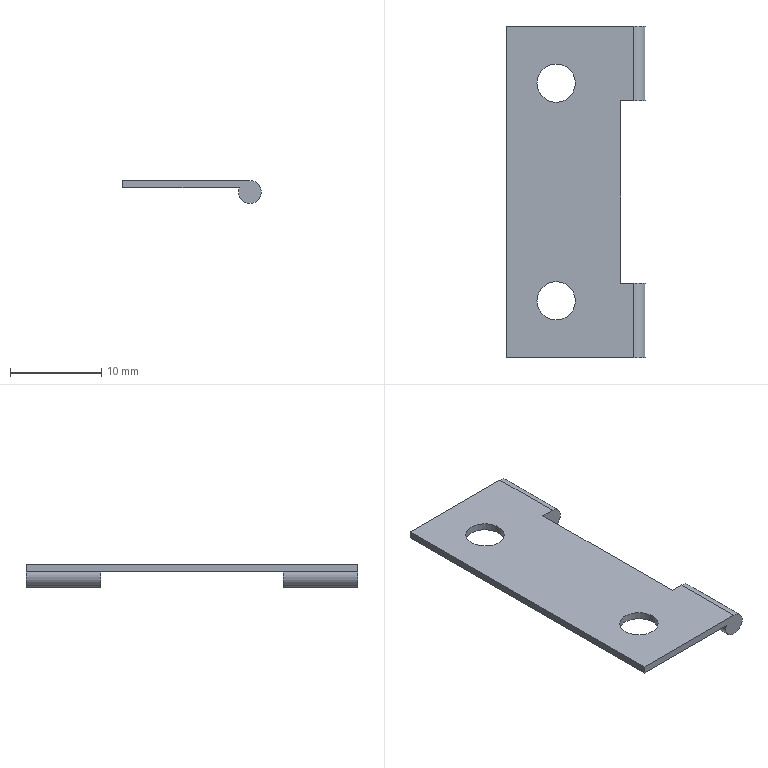Part | STEP file | 1.5 inch micro hinge plate-left | 1 solid | 16 faces | box 15.15 x 36.2 x 2.5 mm | volume 425.73 mm3 | cylinder 8 | plane 8 | commonest cylinder face diameters 2.5 x4 4.2 x4
STEP:
#1=CARTESIAN_POINT('',(0.,0.,0.));
#2=DIRECTION('',(0.,0.,1.));
#3=DIRECTION('',(1.,0.,0.));
#4=AXIS2_PLACEMENT_3D('',#1,#2,#3);
#5=CARTESIAN_POINT('',(-3.65,11.9,0.4));
#6=VERTEX_POINT('',#5);
#7=CARTESIAN_POINT('',(-3.65,11.9,-0.4));
#8=VERTEX_POINT('',#7);
#9=CARTESIAN_POINT('',(-3.65,11.9,-0.4));
#10=DIRECTION('',(0.,0.,-1.));
#11=VECTOR('',#10,1.);
#12=LINE('',#9,#11);
#13=CARTESIAN_POINT('',(-1.55,11.9,-0.4));
#14=DIRECTION('',(0.,0.,-1.));
#15=DIRECTION('',(-1.,0.,0.));
#16=AXIS2_PLACEMENT_3D('',#13,#14,#15);
#17=CYLINDRICAL_SURFACE('',#16,2.1);
#18=CARTESIAN_POINT('',(6.283,0.));
#19=DIRECTION('',(0.,1.));
#20=VECTOR('',#19,1.);
#21=LINE('',#18,#20);
#22=(GEOMETRIC_REPRESENTATION_CONTEXT(2)PARAMETRIC_REPRESENTATION_CONTEXT()REPRESENTATION_CONTEXT('',''));
#23=DEFINITIONAL_REPRESENTATION('',(#21),#22);
#24=PCURVE('',#17,#23);
#25=CARTESIAN_POINT('',(-1.55,11.9,-0.4));
#26=DIRECTION('',(0.,0.,-1.));
#27=DIRECTION('',(-1.,0.,0.));
#28=AXIS2_PLACEMENT_3D('',#25,#26,#27);
#29=CYLINDRICAL_SURFACE('',#28,2.1);
#30=CARTESIAN_POINT('',(0.,0.));
#31=DIRECTION('',(0.,1.));
#32=VECTOR('',#31,1.);
#33=LINE('',#30,#32);
#34=(GEOMETRIC_REPRESENTATION_CONTEXT(2)PARAMETRIC_REPRESENTATION_CONTEXT()REPRESENTATION_CONTEXT('',''));
#35=DEFINITIONAL_REPRESENTATION('',(#33),#34);
#36=PCURVE('',#29,#35);
#37=SURFACE_CURVE('',#12,(#24,#36),.PCURVE_S1.);
#38=EDGE_CURVE('',#6,#8,#37,.T.);
#39=ORIENTED_EDGE('',*,*,#38,.T.);
#40=CARTESIAN_POINT('',(0.55,11.9,-0.4));
#41=VERTEX_POINT('',#40);
#42=CARTESIAN_POINT('',(-1.55,11.9,-0.4));
#43=DIRECTION('',(0.,0.,-1.));
#44=DIRECTION('',(-1.,0.,0.));
#45=AXIS2_PLACEMENT_3D('',#42,#43,#44);
#46=CIRCLE('',#45,2.1);
#47=CARTESIAN_POINT('',(0.,0.));
#48=DIRECTION('',(1.,0.));
#49=VECTOR('',#48,1.);
#50=LINE('',#47,#49);
#51=(GEOMETRIC_REPRESENTATION_CONTEXT(2)PARAMETRIC_REPRESENTATION_CONTEXT()REPRESENTATION_CONTEXT('',''));
#52=DEFINITIONAL_REPRESENTATION('',(#50),#51);
#53=PCURVE('',#17,#52);
#54=CARTESIAN_POINT('',(0.,0.,-0.4));
#55=DIRECTION('',(0.,0.,-1.));
#56=DIRECTION('',(-1.,0.,0.));
#57=AXIS2_PLACEMENT_3D('',#54,#55,#56);
#58=PLANE('',#57);
#59=CARTESIAN_POINT('',(1.55,11.9));
#60=DIRECTION('',(1.,0.));
#61=AXIS2_PLACEMENT_2D('',#59,#60);
#62=CIRCLE('',#61,2.1);
#63=(GEOMETRIC_REPRESENTATION_CONTEXT(2)PARAMETRIC_REPRESENTATION_CONTEXT()REPRESENTATION_CONTEXT('',''));
#64=DEFINITIONAL_REPRESENTATION('',(#62),#63);
#65=PCURVE('',#58,#64);
#66=SURFACE_CURVE('',#46,(#53,#65),.PCURVE_S1.);
#67=EDGE_CURVE('',#41,#8,#66,.T.);
#68=ORIENTED_EDGE('',*,*,#67,.F.);
#69=CARTESIAN_POINT('',(0.55,11.9,0.4));
#70=VERTEX_POINT('',#69);
#71=CARTESIAN_POINT('',(0.55,11.9,-0.4));
#72=DIRECTION('',(0.,0.,-1.));
#73=VECTOR('',#72,1.);
#74=LINE('',#71,#73);
#75=CARTESIAN_POINT('',(3.142,0.));
#76=DIRECTION('',(0.,1.));
#77=VECTOR('',#76,1.);
#78=LINE('',#75,#77);
#79=(GEOMETRIC_REPRESENTATION_CONTEXT(2)PARAMETRIC_REPRESENTATION_CONTEXT()REPRESENTATION_CONTEXT('',''));
#80=DEFINITIONAL_REPRESENTATION('',(#78),#79);
#81=PCURVE('',#17,#80);
#82=CARTESIAN_POINT('',(3.142,0.));
#83=DIRECTION('',(0.,1.));
#84=VECTOR('',#83,1.);
#85=LINE('',#82,#84);
#86=(GEOMETRIC_REPRESENTATION_CONTEXT(2)PARAMETRIC_REPRESENTATION_CONTEXT()REPRESENTATION_CONTEXT('',''));
#87=DEFINITIONAL_REPRESENTATION('',(#85),#86);
#88=PCURVE('',#29,#87);
#89=SURFACE_CURVE('',#74,(#81,#88),.PCURVE_S1.);
#90=EDGE_CURVE('',#70,#41,#89,.T.);
#91=ORIENTED_EDGE('',*,*,#90,.F.);
#92=CARTESIAN_POINT('',(-1.55,11.9,0.4));
#93=DIRECTION('',(0.,0.,-1.));
#94=DIRECTION('',(-1.,0.,0.));
#95=AXIS2_PLACEMENT_3D('',#92,#93,#94);
#96=CIRCLE('',#95,2.1);
#97=CARTESIAN_POINT('',(0.,-0.8));
#98=DIRECTION('',(1.,0.));
#99=VECTOR('',#98,1.);
#100=LINE('',#97,#99);
#101=(GEOMETRIC_REPRESENTATION_CONTEXT(2)PARAMETRIC_REPRESENTATION_CONTEXT()REPRESENTATION_CONTEXT('',''));
#102=DEFINITIONAL_REPRESENTATION('',(#100),#101);
#103=PCURVE('',#17,#102);
#104=CARTESIAN_POINT('',(0.,0.,0.4));
#105=DIRECTION('',(0.,0.,-1.));
#106=DIRECTION('',(-1.,0.,0.));
#107=AXIS2_PLACEMENT_3D('',#104,#105,#106);
#108=PLANE('',#107);
#109=CARTESIAN_POINT('',(1.55,11.9));
#110=DIRECTION('',(1.,0.));
#111=AXIS2_PLACEMENT_2D('',#109,#110);
#112=CIRCLE('',#111,2.1);
#113=(GEOMETRIC_REPRESENTATION_CONTEXT(2)PARAMETRIC_REPRESENTATION_CONTEXT()REPRESENTATION_CONTEXT('',''));
#114=DEFINITIONAL_REPRESENTATION('',(#112),#113);
#115=PCURVE('',#108,#114);
#116=SURFACE_CURVE('',#96,(#103,#115),.PCURVE_S1.);
#117=EDGE_CURVE('',#70,#6,#116,.T.);
#118=ORIENTED_EDGE('',*,*,#117,.T.);
#119=EDGE_LOOP('',(#39,#68,#91,#118));
#120=FACE_BOUND('',#119,.F.);
#121=ADVANCED_FACE('',(#120),#17,.F.);
#122=CARTESIAN_POINT('',(-3.65,-11.9,0.4));
#123=VERTEX_POINT('',#122);
#124=CARTESIAN_POINT('',(-3.65,-11.9,-0.4));
#125=VERTEX_POINT('',#124);
#126=CARTESIAN_POINT('',(-3.65,-11.9,-0.4));
#127=DIRECTION('',(0.,0.,-1.));
#128=VECTOR('',#127,1.);
#129=LINE('',#126,#128);
#130=CARTESIAN_POINT('',(-1.55,-11.9,-0.4));
#131=DIRECTION('',(0.,0.,-1.));
#132=DIRECTION('',(-1.,0.,0.));
#133=AXIS2_PLACEMENT_3D('',#130,#131,#132);
#134=CYLINDRICAL_SURFACE('',#133,2.1);
#135=CARTESIAN_POINT('',(6.283,0.));
#136=DIRECTION('',(0.,1.));
#137=VECTOR('',#136,1.);
#138=LINE('',#135,#137);
#139=(GEOMETRIC_REPRESENTATION_CONTEXT(2)PARAMETRIC_REPRESENTATION_CONTEXT()REPRESENTATION_CONTEXT('',''));
#140=DEFINITIONAL_REPRESENTATION('',(#138),#139);
#141=PCURVE('',#134,#140);
#142=CARTESIAN_POINT('',(-1.55,-11.9,-0.4));
#143=DIRECTION('',(0.,0.,-1.));
#144=DIRECTION('',(-1.,0.,0.));
#145=AXIS2_PLACEMENT_3D('',#142,#143,#144);
#146=CYLINDRICAL_SURFACE('',#145,2.1);
#147=CARTESIAN_POINT('',(0.,0.));
#148=DIRECTION('',(0.,1.));
#149=VECTOR('',#148,1.);
#150=LINE('',#147,#149);
#151=(GEOMETRIC_REPRESENTATION_CONTEXT(2)PARAMETRIC_REPRESENTATION_CONTEXT()REPRESENTATION_CONTEXT('',''));
#152=DEFINITIONAL_REPRESENTATION('',(#150),#151);
#153=PCURVE('',#146,#152);
#154=SURFACE_CURVE('',#129,(#141,#153),.PCURVE_S1.);
#155=EDGE_CURVE('',#123,#125,#154,.T.);
#156=ORIENTED_EDGE('',*,*,#155,.T.);
#157=CARTESIAN_POINT('',(0.55,-11.9,-0.4));
#158=VERTEX_POINT('',#157);
#159=CARTESIAN_POINT('',(-1.55,-11.9,-0.4));
#160=DIRECTION('',(0.,0.,-1.));
#161=DIRECTION('',(-1.,0.,0.));
#162=AXIS2_PLACEMENT_3D('',#159,#160,#161);
#163=CIRCLE('',#162,2.1);
#164=CARTESIAN_POINT('',(0.,0.));
#165=DIRECTION('',(1.,0.));
#166=VECTOR('',#165,1.);
#167=LINE('',#164,#166);
#168=(GEOMETRIC_REPRESENTATION_CONTEXT(2)PARAMETRIC_REPRESENTATION_CONTEXT()REPRESENTATION_CONTEXT('',''));
#169=DEFINITIONAL_REPRESENTATION('',(#167),#168);
#170=PCURVE('',#134,#169);
#171=CARTESIAN_POINT('',(1.55,-11.9));
#172=DIRECTION('',(1.,0.));
#173=AXIS2_PLACEMENT_2D('',#171,#172);
#174=CIRCLE('',#173,2.1);
#175=(GEOMETRIC_REPRESENTATION_CONTEXT(2)PARAMETRIC_REPRESENTATION_CONTEXT()REPRESENTATION_CONTEXT('',''));
#176=DEFINITIONAL_REPRESENTATION('',(#174),#175);
#177=PCURVE('',#58,#176);
#178=SURFACE_CURVE('',#163,(#170,#177),.PCURVE_S1.);
#179=EDGE_CURVE('',#158,#125,#178,.T.);
#180=ORIENTED_EDGE('',*,*,#179,.F.);
#181=CARTESIAN_POINT('',(0.55,-11.9,0.4));
#182=VERTEX_POINT('',#181);
#183=CARTESIAN_POINT('',(0.55,-11.9,-0.4));
#184=DIRECTION('',(0.,0.,-1.));
#185=VECTOR('',#184,1.);
#186=LINE('',#183,#185);
#187=CARTESIAN_POINT('',(3.142,0.));
#188=DIRECTION('',(0.,1.));
#189=VECTOR('',#188,1.);
#190=LINE('',#187,#189);
#191=(GEOMETRIC_REPRESENTATION_CONTEXT(2)PARAMETRIC_REPRESENTATION_CONTEXT()REPRESENTATION_CONTEXT('',''));
#192=DEFINITIONAL_REPRESENTATION('',(#190),#191);
#193=PCURVE('',#134,#192);
#194=CARTESIAN_POINT('',(3.142,0.));
#195=DIRECTION('',(0.,1.));
#196=VECTOR('',#195,1.);
#197=LINE('',#194,#196);
#198=(GEOMETRIC_REPRESENTATION_CONTEXT(2)PARAMETRIC_REPRESENTATION_CONTEXT()REPRESENTATION_CONTEXT('',''));
#199=DEFINITIONAL_REPRESENTATION('',(#197),#198);
#200=PCURVE('',#146,#199);
#201=SURFACE_CURVE('',#186,(#193,#200),.PCURVE_S1.);
#202=EDGE_CURVE('',#182,#158,#201,.T.);
#203=ORIENTED_EDGE('',*,*,#202,.F.);
#204=CARTESIAN_POINT('',(-1.55,-11.9,0.4));
#205=DIRECTION('',(0.,0.,-1.));
#206=DIRECTION('',(-1.,0.,0.));
#207=AXIS2_PLACEMENT_3D('',#204,#205,#206);
#208=CIRCLE('',#207,2.1);
#209=CARTESIAN_POINT('',(0.,-0.8));
#210=DIRECTION('',(1.,0.));
#211=VECTOR('',#210,1.);
#212=LINE('',#209,#211);
#213=(GEOMETRIC_REPRESENTATION_CONTEXT(2)PARAMETRIC_REPRESENTATION_CONTEXT()REPRESENTATION_CONTEXT('',''));
#214=DEFINITIONAL_REPRESENTATION('',(#212),#213);
#215=PCURVE('',#134,#214);
#216=CARTESIAN_POINT('',(1.55,-11.9));
#217=DIRECTION('',(1.,0.));
#218=AXIS2_PLACEMENT_2D('',#216,#217);
#219=CIRCLE('',#218,2.1);
#220=(GEOMETRIC_REPRESENTATION_CONTEXT(2)PARAMETRIC_REPRESENTATION_CONTEXT()REPRESENTATION_CONTEXT('',''));
#221=DEFINITIONAL_REPRESENTATION('',(#219),#220);
#222=PCURVE('',#108,#221);
#223=SURFACE_CURVE('',#208,(#215,#222),.PCURVE_S1.);
#224=EDGE_CURVE('',#182,#123,#223,.T.);
#225=ORIENTED_EDGE('',*,*,#224,.T.);
#226=EDGE_LOOP('',(#156,#180,#203,#225));
#227=FACE_BOUND('',#226,.F.);
#228=ADVANCED_FACE('',(#227),#134,.F.);
#229=CARTESIAN_POINT('',(6.95,18.1,-2.1));
#230=VERTEX_POINT('',#229);
#231=CARTESIAN_POINT('',(5.784,18.1,-0.4));
#232=VERTEX_POINT('',#231);
#233=CARTESIAN_POINT('',(6.95,18.1,-0.85));
#234=DIRECTION('',(0.,1.,0.));
#235=DIRECTION('',(0.,0.,1.));
#236=AXIS2_PLACEMENT_3D('',#233,#234,#235);
#237=CIRCLE('',#236,1.25);
#238=CARTESIAN_POINT('',(6.95,18.1,-0.85));
#239=DIRECTION('',(0.,-1.,0.));
#240=DIRECTION('',(0.,0.,-1.));
#241=AXIS2_PLACEMENT_3D('',#238,#239,#240);
#242=CYLINDRICAL_SURFACE('',#241,1.25);
#243=CARTESIAN_POINT('',(9.425,0.));
#244=DIRECTION('',(-1.,0.));
#245=VECTOR('',#244,1.);
#246=LINE('',#243,#245);
#247=(GEOMETRIC_REPRESENTATION_CONTEXT(2)PARAMETRIC_REPRESENTATION_CONTEXT()REPRESENTATION_CONTEXT('',''));
#248=DEFINITIONAL_REPRESENTATION('',(#246),#247);
#249=PCURVE('',#242,#248);
#250=CARTESIAN_POINT('',(-6.95,18.1,0.4));
#251=DIRECTION('',(0.,-1.,0.));
#252=DIRECTION('',(0.,0.,-1.));
#253=AXIS2_PLACEMENT_3D('',#250,#251,#252);
#254=PLANE('',#253);
#255=CARTESIAN_POINT('',(0.,13.9));
#256=CARTESIAN_POINT('',(0.,16.065));
#257=CARTESIAN_POINT('',(1.875,14.983));
#258=CARTESIAN_POINT('',(3.75,13.9));
#259=CARTESIAN_POINT('',(1.875,12.817));
#260=CARTESIAN_POINT('',(0.,11.735));
#261=CARTESIAN_POINT('',(0.,13.9));
#262=(BOUNDED_CURVE()B_SPLINE_CURVE(2,(#255,#256,#257,#258,#259,#260,#261),.UNSPECIFIED.,.T.,.F.)B_SPLINE_CURVE_WITH_KNOTS((1,2,2,2,2,1),(-2.094,0.,2.094,4.189,6.283,8.378),.UNSPECIFIED.)CURVE()GEOMETRIC_REPRESENTATION_ITEM()RATIONAL_B_SPLINE_CURVE((1.,0.5,1.,0.5,1.,0.5,1.))REPRESENTATION_ITEM(''));
#263=(GEOMETRIC_REPRESENTATION_CONTEXT(2)PARAMETRIC_REPRESENTATION_CONTEXT()REPRESENTATION_CONTEXT('',''));
#264=DEFINITIONAL_REPRESENTATION('',(#262),#263);
#265=PCURVE('',#254,#264);
#266=SURFACE_CURVE('',#237,(#249,#265),.PCURVE_S1.);
#267=EDGE_CURVE('',#230,#232,#266,.T.);
#268=ORIENTED_EDGE('',*,*,#267,.F.);
#269=CARTESIAN_POINT('',(6.95,10.,-2.1));
#270=VERTEX_POINT('',#269);
#271=CARTESIAN_POINT('',(6.95,18.1,-2.1));
#272=DIRECTION('',(0.,-1.,0.));
#273=VECTOR('',#272,1.);
#274=LINE('',#271,#273);
#275=CARTESIAN_POINT('',(6.283,0.));
#276=DIRECTION('',(0.,1.));
#277=VECTOR('',#276,1.);
#278=LINE('',#275,#277);
#279=(GEOMETRIC_REPRESENTATION_CONTEXT(2)PARAMETRIC_REPRESENTATION_CONTEXT()REPRESENTATION_CONTEXT('',''));
#280=DEFINITIONAL_REPRESENTATION('',(#278),#279);
#281=PCURVE('',#242,#280);
#282=CARTESIAN_POINT('',(6.95,18.1,-0.85));
#283=DIRECTION('',(0.,-1.,0.));
#284=DIRECTION('',(0.,0.,-1.));
#285=AXIS2_PLACEMENT_3D('',#282,#283,#284);
#286=CYLINDRICAL_SURFACE('',#285,1.25);
#287=CARTESIAN_POINT('',(0.,0.));
#288=DIRECTION('',(0.,1.));
#289=VECTOR('',#288,1.);
#290=LINE('',#287,#289);
#291=(GEOMETRIC_REPRESENTATION_CONTEXT(2)PARAMETRIC_REPRESENTATION_CONTEXT()REPRESENTATION_CONTEXT('',''));
#292=DEFINITIONAL_REPRESENTATION('',(#290),#291);
#293=PCURVE('',#286,#292);
#294=SURFACE_CURVE('',#274,(#281,#293),.PCURVE_S1.);
#295=EDGE_CURVE('',#230,#270,#294,.T.);
#296=ORIENTED_EDGE('',*,*,#295,.T.);
#297=CARTESIAN_POINT('',(5.784,10.,-0.4));
#298=VERTEX_POINT('',#297);
#299=CARTESIAN_POINT('',(6.95,10.,-0.85));
#300=DIRECTION('',(0.,1.,0.));
#301=DIRECTION('',(0.,0.,1.));
#302=AXIS2_PLACEMENT_3D('',#299,#300,#301);
#303=CIRCLE('',#302,1.25);
#304=CARTESIAN_POINT('',(9.425,8.1));
#305=DIRECTION('',(-1.,0.));
#306=VECTOR('',#305,1.);
#307=LINE('',#304,#306);
#308=(GEOMETRIC_REPRESENTATION_CONTEXT(2)PARAMETRIC_REPRESENTATION_CONTEXT()REPRESENTATION_CONTEXT('',''));
#309=DEFINITIONAL_REPRESENTATION('',(#307),#308);
#310=PCURVE('',#242,#309);
#311=CARTESIAN_POINT('',(5.5,10.,0.4));
#312=DIRECTION('',(0.,1.,0.));
#313=DIRECTION('',(0.,0.,1.));
#314=AXIS2_PLACEMENT_3D('',#311,#312,#313);
#315=PLANE('',#314);
#316=CARTESIAN_POINT('',(-1.25,1.45));
#317=DIRECTION('',(1.,0.));
#318=AXIS2_PLACEMENT_2D('',#316,#317);
#319=CIRCLE('',#318,1.25);
#320=(GEOMETRIC_REPRESENTATION_CONTEXT(2)PARAMETRIC_REPRESENTATION_CONTEXT()REPRESENTATION_CONTEXT('',''));
#321=DEFINITIONAL_REPRESENTATION('',(#319),#320);
#322=PCURVE('',#315,#321);
#323=SURFACE_CURVE('',#303,(#310,#322),.PCURVE_S1.);
#324=EDGE_CURVE('',#270,#298,#323,.T.);
#325=ORIENTED_EDGE('',*,*,#324,.T.);
#326=CARTESIAN_POINT('',(5.784,18.1,-0.4));
#327=DIRECTION('',(0.,-1.,0.));
#328=VECTOR('',#327,1.);
#329=LINE('',#326,#328);
#330=CARTESIAN_POINT('',(4.344,0.));
#331=DIRECTION('',(0.,1.));
#332=VECTOR('',#331,1.);
#333=LINE('',#330,#332);
#334=(GEOMETRIC_REPRESENTATION_CONTEXT(2)PARAMETRIC_REPRESENTATION_CONTEXT()REPRESENTATION_CONTEXT('',''));
#335=DEFINITIONAL_REPRESENTATION('',(#333),#334);
#336=PCURVE('',#242,#335);
#337=CARTESIAN_POINT('',(-5.784,18.1));
#338=DIRECTION('',(0.,-1.));
#339=VECTOR('',#338,1.);
#340=LINE('',#337,#339);
#341=(GEOMETRIC_REPRESENTATION_CONTEXT(2)PARAMETRIC_REPRESENTATION_CONTEXT()REPRESENTATION_CONTEXT('',''));
#342=DEFINITIONAL_REPRESENTATION('',(#340),#341);
#343=PCURVE('',#58,#342);
#344=SURFACE_CURVE('',#329,(#336,#343),.PCURVE_S1.);
#345=EDGE_CURVE('',#232,#298,#344,.T.);
#346=ORIENTED_EDGE('',*,*,#345,.F.);
#347=EDGE_LOOP('',(#268,#296,#325,#346));
#348=FACE_BOUND('',#347,.T.);
#349=ADVANCED_FACE('',(#348),#242,.T.);
#350=CARTESIAN_POINT('',(5.784,-10.,-0.4));
#351=VERTEX_POINT('',#350);
#352=CARTESIAN_POINT('',(6.95,-10.,-2.1));
#353=VERTEX_POINT('',#352);
#354=CARTESIAN_POINT('',(6.95,-10.,-0.85));
#355=DIRECTION('',(0.,-1.,0.));
#356=DIRECTION('',(0.,0.,-1.));
#357=AXIS2_PLACEMENT_3D('',#354,#355,#356);
#358=CIRCLE('',#357,1.25);
#359=CARTESIAN_POINT('',(6.95,18.1,-0.85));
#360=DIRECTION('',(0.,-1.,0.));
#361=DIRECTION('',(0.,0.,-1.));
#362=AXIS2_PLACEMENT_3D('',#359,#360,#361);
#363=CYLINDRICAL_SURFACE('',#362,1.25);
#364=CARTESIAN_POINT('',(0.,28.1));
#365=DIRECTION('',(1.,0.));
#366=VECTOR('',#365,1.);
#367=LINE('',#364,#366);
#368=(GEOMETRIC_REPRESENTATION_CONTEXT(2)PARAMETRIC_REPRESENTATION_CONTEXT()REPRESENTATION_CONTEXT('',''));
#369=DEFINITIONAL_REPRESENTATION('',(#367),#368);
#370=PCURVE('',#363,#369);
#371=CARTESIAN_POINT('',(5.5,-10.,0.4));
#372=DIRECTION('',(0.,-1.,0.));
#373=DIRECTION('',(0.,0.,-1.));
#374=AXIS2_PLACEMENT_3D('',#371,#372,#373);
#375=PLANE('',#374);
#376=CARTESIAN_POINT('',(1.25,1.45));
#377=DIRECTION('',(1.,0.));
#378=AXIS2_PLACEMENT_2D('',#376,#377);
#379=CIRCLE('',#378,1.25);
#380=(GEOMETRIC_REPRESENTATION_CONTEXT(2)PARAMETRIC_REPRESENTATION_CONTEXT()REPRESENTATION_CONTEXT('',''));
#381=DEFINITIONAL_REPRESENTATION('',(#379),#380);
#382=PCURVE('',#375,#381);
#383=SURFACE_CURVE('',#358,(#370,#382),.PCURVE_S1.);
#384=EDGE_CURVE('',#351,#353,#383,.T.);
#385=ORIENTED_EDGE('',*,*,#384,.T.);
#386=CARTESIAN_POINT('',(6.95,-18.1,-2.1));
#387=VERTEX_POINT('',#386);
#388=CARTESIAN_POINT('',(6.95,18.1,-2.1));
#389=DIRECTION('',(0.,-1.,0.));
#390=VECTOR('',#389,1.);
#391=LINE('',#388,#390);
#392=CARTESIAN_POINT('',(6.283,0.));
#393=DIRECTION('',(0.,1.));
#394=VECTOR('',#393,1.);
#395=LINE('',#392,#394);
#396=(GEOMETRIC_REPRESENTATION_CONTEXT(2)PARAMETRIC_REPRESENTATION_CONTEXT()REPRESENTATION_CONTEXT('',''));
#397=DEFINITIONAL_REPRESENTATION('',(#395),#396);
#398=PCURVE('',#363,#397);
#399=CARTESIAN_POINT('',(6.95,18.1,-0.85));
#400=DIRECTION('',(0.,-1.,0.));
#401=DIRECTION('',(0.,0.,-1.));
#402=AXIS2_PLACEMENT_3D('',#399,#400,#401);
#403=CYLINDRICAL_SURFACE('',#402,1.25);
#404=CARTESIAN_POINT('',(0.,0.));
#405=DIRECTION('',(0.,1.));
#406=VECTOR('',#405,1.);
#407=LINE('',#404,#406);
#408=(GEOMETRIC_REPRESENTATION_CONTEXT(2)PARAMETRIC_REPRESENTATION_CONTEXT()REPRESENTATION_CONTEXT('',''));
#409=DEFINITIONAL_REPRESENTATION('',(#407),#408);
#410=PCURVE('',#403,#409);
#411=SURFACE_CURVE('',#391,(#398,#410),.PCURVE_S1.);
#412=EDGE_CURVE('',#353,#387,#411,.T.);
#413=ORIENTED_EDGE('',*,*,#412,.T.);
#414=CARTESIAN_POINT('',(5.784,-18.1,-0.4));
#415=VERTEX_POINT('',#414);
#416=CARTESIAN_POINT('',(6.95,-18.1,-0.85));
#417=DIRECTION('',(0.,1.,0.));
#418=DIRECTION('',(0.,0.,1.));
#419=AXIS2_PLACEMENT_3D('',#416,#417,#418);
#420=CIRCLE('',#419,1.25);
#421=CARTESIAN_POINT('',(9.425,36.2));
#422=DIRECTION('',(-1.,0.));
#423=VECTOR('',#422,1.);
#424=LINE('',#421,#423);
#425=(GEOMETRIC_REPRESENTATION_CONTEXT(2)PARAMETRIC_REPRESENTATION_CONTEXT()REPRESENTATION_CONTEXT('',''));
#426=DEFINITIONAL_REPRESENTATION('',(#424),#425);
#427=PCURVE('',#363,#426);
#428=CARTESIAN_POINT('',(-6.95,-18.1,0.4));
#429=DIRECTION('',(0.,1.,0.));
#430=DIRECTION('',(0.,0.,1.));
#431=AXIS2_PLACEMENT_3D('',#428,#429,#430);
#432=PLANE('',#431);
#433=CARTESIAN_POINT('',(-1.25,13.9));
#434=DIRECTION('',(1.,0.));
#435=AXIS2_PLACEMENT_2D('',#433,#434);
#436=CIRCLE('',#435,1.25);
#437=(GEOMETRIC_REPRESENTATION_CONTEXT(2)PARAMETRIC_REPRESENTATION_CONTEXT()REPRESENTATION_CONTEXT('',''));
#438=DEFINITIONAL_REPRESENTATION('',(#436),#437);
#439=PCURVE('',#432,#438);
#440=SURFACE_CURVE('',#420,(#427,#439),.PCURVE_S1.);
#441=EDGE_CURVE('',#387,#415,#440,.T.);
#442=ORIENTED_EDGE('',*,*,#441,.T.);
#443=CARTESIAN_POINT('',(5.784,18.1,-0.4));
#444=DIRECTION('',(0.,-1.,0.));
#445=VECTOR('',#444,1.);
#446=LINE('',#443,#445);
#447=CARTESIAN_POINT('',(4.344,0.));
#448=DIRECTION('',(0.,1.));
#449=VECTOR('',#448,1.);
#450=LINE('',#447,#449);
#451=(GEOMETRIC_REPRESENTATION_CONTEXT(2)PARAMETRIC_REPRESENTATION_CONTEXT()REPRESENTATION_CONTEXT('',''));
#452=DEFINITIONAL_REPRESENTATION('',(#450),#451);
#453=PCURVE('',#363,#452);
#454=CARTESIAN_POINT('',(-5.784,18.1));
#455=DIRECTION('',(0.,-1.));
#456=VECTOR('',#455,1.);
#457=LINE('',#454,#456);
#458=(GEOMETRIC_REPRESENTATION_CONTEXT(2)PARAMETRIC_REPRESENTATION_CONTEXT()REPRESENTATION_CONTEXT('',''));
#459=DEFINITIONAL_REPRESENTATION('',(#457),#458);
#460=PCURVE('',#58,#459);
#461=SURFACE_CURVE('',#446,(#453,#460),.PCURVE_S1.);
#462=EDGE_CURVE('',#351,#415,#461,.T.);
#463=ORIENTED_EDGE('',*,*,#462,.F.);
#464=EDGE_LOOP('',(#385,#413,#442,#463));
#465=FACE_BOUND('',#464,.T.);
#466=ADVANCED_FACE('',(#465),#363,.T.);
#467=ORIENTED_EDGE('',*,*,#412,.F.);
#468=CARTESIAN_POINT('',(6.95,-10.,0.4));
#469=VERTEX_POINT('',#468);
#470=CARTESIAN_POINT('',(6.95,-10.,-0.85));
#471=DIRECTION('',(0.,-1.,0.));
#472=DIRECTION('',(0.,0.,-1.));
#473=AXIS2_PLACEMENT_3D('',#470,#471,#472);
#474=CIRCLE('',#473,1.25);
#475=CARTESIAN_POINT('',(0.,28.1));
#476=DIRECTION('',(1.,0.));
#477=VECTOR('',#476,1.);
#478=LINE('',#475,#477);
#479=(GEOMETRIC_REPRESENTATION_CONTEXT(2)PARAMETRIC_REPRESENTATION_CONTEXT()REPRESENTATION_CONTEXT('',''));
#480=DEFINITIONAL_REPRESENTATION('',(#478),#479);
#481=PCURVE('',#403,#480);
#482=CARTESIAN_POINT('',(1.25,1.45));
#483=DIRECTION('',(1.,0.));
#484=AXIS2_PLACEMENT_2D('',#482,#483);
#485=CIRCLE('',#484,1.25);
#486=(GEOMETRIC_REPRESENTATION_CONTEXT(2)PARAMETRIC_REPRESENTATION_CONTEXT()REPRESENTATION_CONTEXT('',''));
#487=DEFINITIONAL_REPRESENTATION('',(#485),#486);
#488=PCURVE('',#375,#487);
#489=SURFACE_CURVE('',#474,(#481,#488),.PCURVE_S1.);
#490=EDGE_CURVE('',#353,#469,#489,.T.);
#491=ORIENTED_EDGE('',*,*,#490,.T.);
#492=CARTESIAN_POINT('',(6.95,-18.1,0.4));
#493=VERTEX_POINT('',#492);
#494=CARTESIAN_POINT('',(6.95,-18.1,0.4));
#495=DIRECTION('',(0.,1.,0.));
#496=VECTOR('',#495,1.);
#497=LINE('',#494,#496);
#498=CARTESIAN_POINT('',(3.142,36.2));
#499=DIRECTION('',(0.,-1.));
#500=VECTOR('',#499,1.);
#501=LINE('',#498,#500);
#502=(GEOMETRIC_REPRESENTATION_CONTEXT(2)PARAMETRIC_REPRESENTATION_CONTEXT()REPRESENTATION_CONTEXT('',''));
#503=DEFINITIONAL_REPRESENTATION('',(#501),#502);
#504=PCURVE('',#403,#503);
#505=CARTESIAN_POINT('',(-6.95,-18.1));
#506=DIRECTION('',(0.,1.));
#507=VECTOR('',#506,1.);
#508=LINE('',#505,#507);
#509=(GEOMETRIC_REPRESENTATION_CONTEXT(2)PARAMETRIC_REPRESENTATION_CONTEXT()REPRESENTATION_CONTEXT('',''));
#510=DEFINITIONAL_REPRESENTATION('',(#508),#509);
#511=PCURVE('',#108,#510);
#512=SURFACE_CURVE('',#497,(#504,#511),.PCURVE_S1.);
#513=EDGE_CURVE('',#493,#469,#512,.T.);
#514=ORIENTED_EDGE('',*,*,#513,.F.);
#515=CARTESIAN_POINT('',(6.95,-18.1,-0.85));
#516=DIRECTION('',(0.,1.,0.));
#517=DIRECTION('',(0.,0.,1.));
#518=AXIS2_PLACEMENT_3D('',#515,#516,#517);
#519=CIRCLE('',#518,1.25);
#520=CARTESIAN_POINT('',(3.142,36.2));
#521=DIRECTION('',(-1.,0.));
#522=VECTOR('',#521,1.);
#523=LINE('',#520,#522);
#524=(GEOMETRIC_REPRESENTATION_CONTEXT(2)PARAMETRIC_REPRESENTATION_CONTEXT()REPRESENTATION_CONTEXT('',''));
#525=DEFINITIONAL_REPRESENTATION('',(#523),#524);
#526=PCURVE('',#403,#525);
#527=CARTESIAN_POINT('',(-1.25,13.9));
#528=DIRECTION('',(1.,0.));
#529=AXIS2_PLACEMENT_2D('',#527,#528);
#530=CIRCLE('',#529,1.25);
#531=(GEOMETRIC_REPRESENTATION_CONTEXT(2)PARAMETRIC_REPRESENTATION_CONTEXT()REPRESENTATION_CONTEXT('',''));
#532=DEFINITIONAL_REPRESENTATION('',(#530),#531);
#533=PCURVE('',#432,#532);
#534=SURFACE_CURVE('',#519,(#526,#533),.PCURVE_S1.);
#535=EDGE_CURVE('',#493,#387,#534,.T.);
#536=ORIENTED_EDGE('',*,*,#535,.T.);
#537=EDGE_LOOP('',(#467,#491,#514,#536));
#538=FACE_BOUND('',#537,.T.);
#539=ADVANCED_FACE('',(#538),#403,.T.);
#540=CARTESIAN_POINT('',(5.5,-10.,-0.4));
#541=VERTEX_POINT('',#540);
#542=CARTESIAN_POINT('',(0.,-10.,-0.4));
#543=DIRECTION('',(-1.,0.,0.));
#544=VECTOR('',#543,1.);
#545=LINE('',#542,#544);
#546=CARTESIAN_POINT('',(0.,-10.));
#547=DIRECTION('',(1.,0.));
#548=VECTOR('',#547,1.);
#549=LINE('',#546,#548);
#550=(GEOMETRIC_REPRESENTATION_CONTEXT(2)PARAMETRIC_REPRESENTATION_CONTEXT()REPRESENTATION_CONTEXT('',''));
#551=DEFINITIONAL_REPRESENTATION('',(#549),#550);
#552=PCURVE('',#58,#551);
#553=CARTESIAN_POINT('',(0.8,-5.5));
#554=DIRECTION('',(0.,-1.));
#555=VECTOR('',#554,1.);
#556=LINE('',#553,#555);
#557=(GEOMETRIC_REPRESENTATION_CONTEXT(2)PARAMETRIC_REPRESENTATION_CONTEXT()REPRESENTATION_CONTEXT('',''));
#558=DEFINITIONAL_REPRESENTATION('',(#556),#557);
#559=PCURVE('',#375,#558);
#560=SURFACE_CURVE('',#545,(#552,#559),.PCURVE_S1.);
#561=EDGE_CURVE('',#351,#541,#560,.T.);
#562=ORIENTED_EDGE('',*,*,#561,.F.);
#563=ORIENTED_EDGE('',*,*,#462,.T.);
#564=CARTESIAN_POINT('',(-6.95,-18.1,-0.4));
#565=VERTEX_POINT('',#564);
#566=CARTESIAN_POINT('',(-6.95,-18.1,-0.4));
#567=DIRECTION('',(1.,0.,0.));
#568=VECTOR('',#567,1.);
#569=LINE('',#566,#568);
#570=CARTESIAN_POINT('',(6.95,-18.1));
#571=DIRECTION('',(-1.,0.));
#572=VECTOR('',#571,1.);
#573=LINE('',#570,#572);
#574=(GEOMETRIC_REPRESENTATION_CONTEXT(2)PARAMETRIC_REPRESENTATION_CONTEXT()REPRESENTATION_CONTEXT('',''));
#575=DEFINITIONAL_REPRESENTATION('',(#573),#574);
#576=PCURVE('',#58,#575);
#577=CARTESIAN_POINT('',(-0.8,0.));
#578=DIRECTION('',(0.,1.));
#579=VECTOR('',#578,1.);
#580=LINE('',#577,#579);
#581=(GEOMETRIC_REPRESENTATION_CONTEXT(2)PARAMETRIC_REPRESENTATION_CONTEXT()REPRESENTATION_CONTEXT('',''));
#582=DEFINITIONAL_REPRESENTATION('',(#580),#581);
#583=PCURVE('',#432,#582);
#584=SURFACE_CURVE('',#569,(#576,#583),.PCURVE_S1.);
#585=EDGE_CURVE('',#565,#415,#584,.T.);
#586=ORIENTED_EDGE('',*,*,#585,.F.);
#587=CARTESIAN_POINT('',(-6.95,18.1,-0.4));
#588=VERTEX_POINT('',#587);
#589=CARTESIAN_POINT('',(-6.95,-18.1,-0.4));
#590=DIRECTION('',(0.,-1.,0.));
#591=VECTOR('',#590,1.);
#592=LINE('',#589,#591);
#593=CARTESIAN_POINT('',(6.95,-18.1));
#594=DIRECTION('',(0.,-1.));
#595=VECTOR('',#594,1.);
#596=LINE('',#593,#595);
#597=(GEOMETRIC_REPRESENTATION_CONTEXT(2)PARAMETRIC_REPRESENTATION_CONTEXT()REPRESENTATION_CONTEXT('',''));
#598=DEFINITIONAL_REPRESENTATION('',(#596),#597);
#599=PCURVE('',#58,#598);
#600=CARTESIAN_POINT('',(-6.95,-18.1,0.4));
#601=DIRECTION('',(1.,0.,0.));
#602=DIRECTION('',(0.,0.,-1.));
#603=AXIS2_PLACEMENT_3D('',#600,#601,#602);
#604=PLANE('',#603);
#605=CARTESIAN_POINT('',(0.8,0.));
#606=DIRECTION('',(0.,-1.));
#607=VECTOR('',#606,1.);
#608=LINE('',#605,#607);
#609=(GEOMETRIC_REPRESENTATION_CONTEXT(2)PARAMETRIC_REPRESENTATION_CONTEXT()REPRESENTATION_CONTEXT('',''));
#610=DEFINITIONAL_REPRESENTATION('',(#608),#609);
#611=PCURVE('',#604,#610);
#612=SURFACE_CURVE('',#592,(#599,#611),.PCURVE_S1.);
#613=EDGE_CURVE('',#588,#565,#612,.T.);
#614=ORIENTED_EDGE('',*,*,#613,.F.);
#615=CARTESIAN_POINT('',(-6.95,18.1,-0.4));
#616=DIRECTION('',(-1.,0.,0.));
#617=VECTOR('',#616,1.);
#618=LINE('',#615,#617);
#619=CARTESIAN_POINT('',(6.95,18.1));
#620=DIRECTION('',(1.,0.));
#621=VECTOR('',#620,1.);
#622=LINE('',#619,#621);
#623=(GEOMETRIC_REPRESENTATION_CONTEXT(2)PARAMETRIC_REPRESENTATION_CONTEXT()REPRESENTATION_CONTEXT('',''));
#624=DEFINITIONAL_REPRESENTATION('',(#622),#623);
#625=PCURVE('',#58,#624);
#626=CARTESIAN_POINT('',(0.8,0.));
#627=DIRECTION('',(0.,-1.));
#628=VECTOR('',#627,1.);
#629=LINE('',#626,#628);
#630=(GEOMETRIC_REPRESENTATION_CONTEXT(2)PARAMETRIC_REPRESENTATION_CONTEXT()REPRESENTATION_CONTEXT('',''));
#631=DEFINITIONAL_REPRESENTATION('',(#629),#630);
#632=PCURVE('',#254,#631);
#633=SURFACE_CURVE('',#618,(#625,#632),.PCURVE_S1.);
#634=EDGE_CURVE('',#232,#588,#633,.T.);
#635=ORIENTED_EDGE('',*,*,#634,.F.);
#636=ORIENTED_EDGE('',*,*,#345,.T.);
#637=CARTESIAN_POINT('',(5.5,10.,-0.4));
#638=VERTEX_POINT('',#637);
#639=CARTESIAN_POINT('',(0.,10.,-0.4));
#640=DIRECTION('',(1.,0.,0.));
#641=VECTOR('',#640,1.);
#642=LINE('',#639,#641);
#643=CARTESIAN_POINT('',(0.,10.));
#644=DIRECTION('',(-1.,0.));
#645=VECTOR('',#644,1.);
#646=LINE('',#643,#645);
#647=(GEOMETRIC_REPRESENTATION_CONTEXT(2)PARAMETRIC_REPRESENTATION_CONTEXT()REPRESENTATION_CONTEXT('',''));
#648=DEFINITIONAL_REPRESENTATION('',(#646),#647);
#649=PCURVE('',#58,#648);
#650=CARTESIAN_POINT('',(-0.8,-5.5));
#651=DIRECTION('',(0.,1.));
#652=VECTOR('',#651,1.);
#653=LINE('',#650,#652);
#654=(GEOMETRIC_REPRESENTATION_CONTEXT(2)PARAMETRIC_REPRESENTATION_CONTEXT()REPRESENTATION_CONTEXT('',''));
#655=DEFINITIONAL_REPRESENTATION('',(#653),#654);
#656=PCURVE('',#315,#655);
#657=SURFACE_CURVE('',#642,(#649,#656),.PCURVE_S1.);
#658=EDGE_CURVE('',#638,#298,#657,.T.);
#659=ORIENTED_EDGE('',*,*,#658,.F.);
#660=CARTESIAN_POINT('',(5.5,0.,-0.4));
#661=DIRECTION('',(0.,1.,0.));
#662=VECTOR('',#661,1.);
#663=LINE('',#660,#662);
#664=CARTESIAN_POINT('',(-5.5,0.));
#665=DIRECTION('',(0.,1.));
#666=VECTOR('',#665,1.);
#667=LINE('',#664,#666);
#668=(GEOMETRIC_REPRESENTATION_CONTEXT(2)PARAMETRIC_REPRESENTATION_CONTEXT()REPRESENTATION_CONTEXT('',''));
#669=DEFINITIONAL_REPRESENTATION('',(#667),#668);
#670=PCURVE('',#58,#669);
#671=CARTESIAN_POINT('',(5.5,0.,0.));
#672=DIRECTION('',(-1.,0.,0.));
#673=DIRECTION('',(0.,0.,1.));
#674=AXIS2_PLACEMENT_3D('',#671,#672,#673);
#675=PLANE('',#674);
#676=CARTESIAN_POINT('',(-0.4,0.));
#677=DIRECTION('',(0.,1.));
#678=VECTOR('',#677,1.);
#679=LINE('',#676,#678);
#680=(GEOMETRIC_REPRESENTATION_CONTEXT(2)PARAMETRIC_REPRESENTATION_CONTEXT()REPRESENTATION_CONTEXT('',''));
#681=DEFINITIONAL_REPRESENTATION('',(#679),#680);
#682=PCURVE('',#675,#681);
#683=SURFACE_CURVE('',#663,(#670,#682),.PCURVE_S1.);
#684=EDGE_CURVE('',#541,#638,#683,.T.);
#685=ORIENTED_EDGE('',*,*,#684,.F.);
#686=EDGE_LOOP('',(#562,#563,#586,#614,#635,#636,#659,#685));
#687=FACE_BOUND('',#686,.T.);
#688=CARTESIAN_POINT('',(-1.55,11.9,-0.4));
#689=DIRECTION('',(0.,0.,-1.));
#690=DIRECTION('',(-1.,0.,0.));
#691=AXIS2_PLACEMENT_3D('',#688,#689,#690);
#692=CIRCLE('',#691,2.1);
#693=CARTESIAN_POINT('',(1.55,11.9));
#694=DIRECTION('',(1.,0.));
#695=AXIS2_PLACEMENT_2D('',#693,#694);
#696=CIRCLE('',#695,2.1);
#697=(GEOMETRIC_REPRESENTATION_CONTEXT(2)PARAMETRIC_REPRESENTATION_CONTEXT()REPRESENTATION_CONTEXT('',''));
#698=DEFINITIONAL_REPRESENTATION('',(#696),#697);
#699=PCURVE('',#58,#698);
#700=CARTESIAN_POINT('',(0.,0.));
#701=DIRECTION('',(1.,0.));
#702=VECTOR('',#701,1.);
#703=LINE('',#700,#702);
#704=(GEOMETRIC_REPRESENTATION_CONTEXT(2)PARAMETRIC_REPRESENTATION_CONTEXT()REPRESENTATION_CONTEXT('',''));
#705=DEFINITIONAL_REPRESENTATION('',(#703),#704);
#706=PCURVE('',#29,#705);
#707=SURFACE_CURVE('',#692,(#699,#706),.PCURVE_S1.);
#708=EDGE_CURVE('',#8,#41,#707,.T.);
#709=ORIENTED_EDGE('',*,*,#708,.F.);
#710=ORIENTED_EDGE('',*,*,#67,.F.);
#711=EDGE_LOOP('',(#709,#710));
#712=FACE_BOUND('',#711,.T.);
#713=CARTESIAN_POINT('',(-1.55,-11.9,-0.4));
#714=DIRECTION('',(0.,0.,-1.));
#715=DIRECTION('',(-1.,0.,0.));
#716=AXIS2_PLACEMENT_3D('',#713,#714,#715);
#717=CIRCLE('',#716,2.1);
#718=CARTESIAN_POINT('',(1.55,-11.9));
#719=DIRECTION('',(1.,0.));
#720=AXIS2_PLACEMENT_2D('',#718,#719);
#721=CIRCLE('',#720,2.1);
#722=(GEOMETRIC_REPRESENTATION_CONTEXT(2)PARAMETRIC_REPRESENTATION_CONTEXT()REPRESENTATION_CONTEXT('',''));
#723=DEFINITIONAL_REPRESENTATION('',(#721),#722);
#724=PCURVE('',#58,#723);
#725=CARTESIAN_POINT('',(0.,0.));
#726=DIRECTION('',(1.,0.));
#727=VECTOR('',#726,1.);
#728=LINE('',#725,#727);
#729=(GEOMETRIC_REPRESENTATION_CONTEXT(2)PARAMETRIC_REPRESENTATION_CONTEXT()REPRESENTATION_CONTEXT('',''));
#730=DEFINITIONAL_REPRESENTATION('',(#728),#729);
#731=PCURVE('',#146,#730);
#732=SURFACE_CURVE('',#717,(#724,#731),.PCURVE_S1.);
#733=EDGE_CURVE('',#125,#158,#732,.T.);
#734=ORIENTED_EDGE('',*,*,#733,.F.);
#735=ORIENTED_EDGE('',*,*,#179,.F.);
#736=EDGE_LOOP('',(#734,#735));
#737=FACE_BOUND('',#736,.T.);
#738=ADVANCED_FACE('',(#687,#712,#737),#58,.T.);
#739=CARTESIAN_POINT('',(6.95,18.1,0.4));
#740=VERTEX_POINT('',#739);
#741=CARTESIAN_POINT('',(-6.95,18.1,0.4));
#742=VERTEX_POINT('',#741);
#743=CARTESIAN_POINT('',(-6.95,18.1,0.4));
#744=DIRECTION('',(-1.,0.,0.));
#745=VECTOR('',#744,1.);
#746=LINE('',#743,#745);
#747=CARTESIAN_POINT('',(0.,0.));
#748=DIRECTION('',(0.,-1.));
#749=VECTOR('',#748,1.);
#750=LINE('',#747,#749);
#751=(GEOMETRIC_REPRESENTATION_CONTEXT(2)PARAMETRIC_REPRESENTATION_CONTEXT()REPRESENTATION_CONTEXT('',''));
#752=DEFINITIONAL_REPRESENTATION('',(#750),#751);
#753=PCURVE('',#254,#752);
#754=CARTESIAN_POINT('',(6.95,18.1));
#755=DIRECTION('',(1.,0.));
#756=VECTOR('',#755,1.);
#757=LINE('',#754,#756);
#758=(GEOMETRIC_REPRESENTATION_CONTEXT(2)PARAMETRIC_REPRESENTATION_CONTEXT()REPRESENTATION_CONTEXT('',''));
#759=DEFINITIONAL_REPRESENTATION('',(#757),#758);
#760=PCURVE('',#108,#759);
#761=SURFACE_CURVE('',#746,(#753,#760),.PCURVE_S1.);
#762=EDGE_CURVE('',#740,#742,#761,.T.);
#763=ORIENTED_EDGE('',*,*,#762,.F.);
#764=CARTESIAN_POINT('',(6.95,18.1,-0.85));
#765=DIRECTION('',(0.,1.,0.));
#766=DIRECTION('',(0.,0.,1.));
#767=AXIS2_PLACEMENT_3D('',#764,#765,#766);
#768=CIRCLE('',#767,1.25);
#769=CARTESIAN_POINT('',(0.,13.9));
#770=CARTESIAN_POINT('',(0.,16.065));
#771=CARTESIAN_POINT('',(1.875,14.983));
#772=CARTESIAN_POINT('',(3.75,13.9));
#773=CARTESIAN_POINT('',(1.875,12.817));
#774=CARTESIAN_POINT('',(0.,11.735));
#775=CARTESIAN_POINT('',(0.,13.9));
#776=(BOUNDED_CURVE()B_SPLINE_CURVE(2,(#769,#770,#771,#772,#773,#774,#775),.UNSPECIFIED.,.T.,.F.)B_SPLINE_CURVE_WITH_KNOTS((1,2,2,2,2,1),(-2.094,0.,2.094,4.189,6.283,8.378),.UNSPECIFIED.)CURVE()GEOMETRIC_REPRESENTATION_ITEM()RATIONAL_B_SPLINE_CURVE((1.,0.5,1.,0.5,1.,0.5,1.))REPRESENTATION_ITEM(''));
#777=(GEOMETRIC_REPRESENTATION_CONTEXT(2)PARAMETRIC_REPRESENTATION_CONTEXT()REPRESENTATION_CONTEXT('',''));
#778=DEFINITIONAL_REPRESENTATION('',(#776),#777);
#779=PCURVE('',#254,#778);
#780=CARTESIAN_POINT('',(3.142,0.));
#781=DIRECTION('',(-1.,0.));
#782=VECTOR('',#781,1.);
#783=LINE('',#780,#782);
#784=(GEOMETRIC_REPRESENTATION_CONTEXT(2)PARAMETRIC_REPRESENTATION_CONTEXT()REPRESENTATION_CONTEXT('',''));
#785=DEFINITIONAL_REPRESENTATION('',(#783),#784);
#786=PCURVE('',#286,#785);
#787=SURFACE_CURVE('',#768,(#779,#786),.PCURVE_S1.);
#788=EDGE_CURVE('',#740,#230,#787,.T.);
#789=ORIENTED_EDGE('',*,*,#788,.T.);
#790=ORIENTED_EDGE('',*,*,#267,.T.);
#791=ORIENTED_EDGE('',*,*,#634,.T.);
#792=CARTESIAN_POINT('',(-6.95,18.1,0.4));
#793=DIRECTION('',(0.,0.,-1.));
#794=VECTOR('',#793,1.);
#795=LINE('',#792,#794);
#796=CARTESIAN_POINT('',(0.,0.));
#797=DIRECTION('',(1.,0.));
#798=VECTOR('',#797,1.);
#799=LINE('',#796,#798);
#800=(GEOMETRIC_REPRESENTATION_CONTEXT(2)PARAMETRIC_REPRESENTATION_CONTEXT()REPRESENTATION_CONTEXT('',''));
#801=DEFINITIONAL_REPRESENTATION('',(#799),#800);
#802=PCURVE('',#254,#801);
#803=CARTESIAN_POINT('',(0.,36.2));
#804=DIRECTION('',(1.,0.));
#805=VECTOR('',#804,1.);
#806=LINE('',#803,#805);
#807=(GEOMETRIC_REPRESENTATION_CONTEXT(2)PARAMETRIC_REPRESENTATION_CONTEXT()REPRESENTATION_CONTEXT('',''));
#808=DEFINITIONAL_REPRESENTATION('',(#806),#807);
#809=PCURVE('',#604,#808);
#810=SURFACE_CURVE('',#795,(#802,#809),.PCURVE_S1.);
#811=EDGE_CURVE('',#742,#588,#810,.T.);
#812=ORIENTED_EDGE('',*,*,#811,.F.);
#813=EDGE_LOOP('',(#763,#789,#790,#791,#812));
#814=FACE_BOUND('',#813,.T.);
#815=ADVANCED_FACE('',(#814),#254,.F.);
#816=ORIENTED_EDGE('',*,*,#613,.T.);
#817=CARTESIAN_POINT('',(-6.95,-18.1,0.4));
#818=VERTEX_POINT('',#817);
#819=CARTESIAN_POINT('',(-6.95,-18.1,0.4));
#820=DIRECTION('',(0.,0.,-1.));
#821=VECTOR('',#820,1.);
#822=LINE('',#819,#821);
#823=CARTESIAN_POINT('',(0.,0.));
#824=DIRECTION('',(1.,0.));
#825=VECTOR('',#824,1.);
#826=LINE('',#823,#825);
#827=(GEOMETRIC_REPRESENTATION_CONTEXT(2)PARAMETRIC_REPRESENTATION_CONTEXT()REPRESENTATION_CONTEXT('',''));
#828=DEFINITIONAL_REPRESENTATION('',(#826),#827);
#829=PCURVE('',#604,#828);
#830=CARTESIAN_POINT('',(0.,0.));
#831=DIRECTION('',(-1.,0.));
#832=VECTOR('',#831,1.);
#833=LINE('',#830,#832);
#834=(GEOMETRIC_REPRESENTATION_CONTEXT(2)PARAMETRIC_REPRESENTATION_CONTEXT()REPRESENTATION_CONTEXT('',''));
#835=DEFINITIONAL_REPRESENTATION('',(#833),#834);
#836=PCURVE('',#432,#835);
#837=SURFACE_CURVE('',#822,(#829,#836),.PCURVE_S1.);
#838=EDGE_CURVE('',#818,#565,#837,.T.);
#839=ORIENTED_EDGE('',*,*,#838,.F.);
#840=CARTESIAN_POINT('',(-6.95,-18.1,0.4));
#841=DIRECTION('',(0.,-1.,0.));
#842=VECTOR('',#841,1.);
#843=LINE('',#840,#842);
#844=CARTESIAN_POINT('',(0.,0.));
#845=DIRECTION('',(0.,-1.));
#846=VECTOR('',#845,1.);
#847=LINE('',#844,#846);
#848=(GEOMETRIC_REPRESENTATION_CONTEXT(2)PARAMETRIC_REPRESENTATION_CONTEXT()REPRESENTATION_CONTEXT('',''));
#849=DEFINITIONAL_REPRESENTATION('',(#847),#848);
#850=PCURVE('',#604,#849);
#851=CARTESIAN_POINT('',(6.95,-18.1));
#852=DIRECTION('',(0.,-1.));
#853=VECTOR('',#852,1.);
#854=LINE('',#851,#853);
#855=(GEOMETRIC_REPRESENTATION_CONTEXT(2)PARAMETRIC_REPRESENTATION_CONTEXT()REPRESENTATION_CONTEXT('',''));
#856=DEFINITIONAL_REPRESENTATION('',(#854),#855);
#857=PCURVE('',#108,#856);
#858=SURFACE_CURVE('',#843,(#850,#857),.PCURVE_S1.);
#859=EDGE_CURVE('',#742,#818,#858,.T.);
#860=ORIENTED_EDGE('',*,*,#859,.F.);
#861=ORIENTED_EDGE('',*,*,#811,.T.);
#862=EDGE_LOOP('',(#816,#839,#860,#861));
#863=FACE_BOUND('',#862,.T.);
#864=ADVANCED_FACE('',(#863),#604,.F.);
#865=ORIENTED_EDGE('',*,*,#585,.T.);
#866=ORIENTED_EDGE('',*,*,#441,.F.);
#867=ORIENTED_EDGE('',*,*,#535,.F.);
#868=CARTESIAN_POINT('',(-6.95,-18.1,0.4));
#869=DIRECTION('',(1.,0.,0.));
#870=VECTOR('',#869,1.);
#871=LINE('',#868,#870);
#872=CARTESIAN_POINT('',(0.,0.));
#873=DIRECTION('',(0.,1.));
#874=VECTOR('',#873,1.);
#875=LINE('',#872,#874);
#876=(GEOMETRIC_REPRESENTATION_CONTEXT(2)PARAMETRIC_REPRESENTATION_CONTEXT()REPRESENTATION_CONTEXT('',''));
#877=DEFINITIONAL_REPRESENTATION('',(#875),#876);
#878=PCURVE('',#432,#877);
#879=CARTESIAN_POINT('',(6.95,-18.1));
#880=DIRECTION('',(-1.,0.));
#881=VECTOR('',#880,1.);
#882=LINE('',#879,#881);
#883=(GEOMETRIC_REPRESENTATION_CONTEXT(2)PARAMETRIC_REPRESENTATION_CONTEXT()REPRESENTATION_CONTEXT('',''));
#884=DEFINITIONAL_REPRESENTATION('',(#882),#883);
#885=PCURVE('',#108,#884);
#886=SURFACE_CURVE('',#871,(#878,#885),.PCURVE_S1.);
#887=EDGE_CURVE('',#818,#493,#886,.T.);
#888=ORIENTED_EDGE('',*,*,#887,.F.);
#889=ORIENTED_EDGE('',*,*,#838,.T.);
#890=EDGE_LOOP('',(#865,#866,#867,#888,#889));
#891=FACE_BOUND('',#890,.T.);
#892=ADVANCED_FACE('',(#891),#432,.F.);
#893=ORIENTED_EDGE('',*,*,#513,.T.);
#894=CARTESIAN_POINT('',(5.5,-10.,0.4));
#895=VERTEX_POINT('',#894);
#896=CARTESIAN_POINT('',(5.5,-10.,0.4));
#897=DIRECTION('',(1.,0.,0.));
#898=VECTOR('',#897,1.);
#899=LINE('',#896,#898);
#900=CARTESIAN_POINT('',(-5.5,-10.));
#901=DIRECTION('',(-1.,0.));
#902=VECTOR('',#901,1.);
#903=LINE('',#900,#902);
#904=(GEOMETRIC_REPRESENTATION_CONTEXT(2)PARAMETRIC_REPRESENTATION_CONTEXT()REPRESENTATION_CONTEXT('',''));
#905=DEFINITIONAL_REPRESENTATION('',(#903),#904);
#906=PCURVE('',#108,#905);
#907=CARTESIAN_POINT('',(0.,0.));
#908=DIRECTION('',(0.,1.));
#909=VECTOR('',#908,1.);
#910=LINE('',#907,#909);
#911=(GEOMETRIC_REPRESENTATION_CONTEXT(2)PARAMETRIC_REPRESENTATION_CONTEXT()REPRESENTATION_CONTEXT('',''));
#912=DEFINITIONAL_REPRESENTATION('',(#910),#911);
#913=PCURVE('',#375,#912);
#914=SURFACE_CURVE('',#899,(#906,#913),.PCURVE_S1.);
#915=EDGE_CURVE('',#895,#469,#914,.T.);
#916=ORIENTED_EDGE('',*,*,#915,.F.);
#917=CARTESIAN_POINT('',(5.5,10.,0.4));
#918=VERTEX_POINT('',#917);
#919=CARTESIAN_POINT('',(5.5,-10.,0.4));
#920=DIRECTION('',(0.,-1.,0.));
#921=VECTOR('',#920,1.);
#922=LINE('',#919,#921);
#923=CARTESIAN_POINT('',(-5.5,-10.));
#924=DIRECTION('',(0.,-1.));
#925=VECTOR('',#924,1.);
#926=LINE('',#923,#925);
#927=(GEOMETRIC_REPRESENTATION_CONTEXT(2)PARAMETRIC_REPRESENTATION_CONTEXT()REPRESENTATION_CONTEXT('',''));
#928=DEFINITIONAL_REPRESENTATION('',(#926),#927);
#929=PCURVE('',#108,#928);
#930=CARTESIAN_POINT('',(0.4,-10.));
#931=DIRECTION('',(0.,-1.));
#932=VECTOR('',#931,1.);
#933=LINE('',#930,#932);
#934=(GEOMETRIC_REPRESENTATION_CONTEXT(2)PARAMETRIC_REPRESENTATION_CONTEXT()REPRESENTATION_CONTEXT('',''));
#935=DEFINITIONAL_REPRESENTATION('',(#933),#934);
#936=PCURVE('',#675,#935);
#937=SURFACE_CURVE('',#922,(#929,#936),.PCURVE_S1.);
#938=EDGE_CURVE('',#918,#895,#937,.T.);
#939=ORIENTED_EDGE('',*,*,#938,.F.);
#940=CARTESIAN_POINT('',(6.95,10.,0.4));
#941=VERTEX_POINT('',#940);
#942=CARTESIAN_POINT('',(5.5,10.,0.4));
#943=DIRECTION('',(1.,0.,0.));
#944=VECTOR('',#943,1.);
#945=LINE('',#942,#944);
#946=CARTESIAN_POINT('',(-5.5,10.));
#947=DIRECTION('',(-1.,0.));
#948=VECTOR('',#947,1.);
#949=LINE('',#946,#948);
#950=(GEOMETRIC_REPRESENTATION_CONTEXT(2)PARAMETRIC_REPRESENTATION_CONTEXT()REPRESENTATION_CONTEXT('',''));
#951=DEFINITIONAL_REPRESENTATION('',(#949),#950);
#952=PCURVE('',#108,#951);
#953=CARTESIAN_POINT('',(0.,0.));
#954=DIRECTION('',(0.,1.));
#955=VECTOR('',#954,1.);
#956=LINE('',#953,#955);
#957=(GEOMETRIC_REPRESENTATION_CONTEXT(2)PARAMETRIC_REPRESENTATION_CONTEXT()REPRESENTATION_CONTEXT('',''));
#958=DEFINITIONAL_REPRESENTATION('',(#956),#957);
#959=PCURVE('',#315,#958);
#960=SURFACE_CURVE('',#945,(#952,#959),.PCURVE_S1.);
#961=EDGE_CURVE('',#918,#941,#960,.T.);
#962=ORIENTED_EDGE('',*,*,#961,.T.);
#963=CARTESIAN_POINT('',(6.95,-18.1,0.4));
#964=DIRECTION('',(0.,1.,0.));
#965=VECTOR('',#964,1.);
#966=LINE('',#963,#965);
#967=CARTESIAN_POINT('',(-6.95,-18.1));
#968=DIRECTION('',(0.,1.));
#969=VECTOR('',#968,1.);
#970=LINE('',#967,#969);
#971=(GEOMETRIC_REPRESENTATION_CONTEXT(2)PARAMETRIC_REPRESENTATION_CONTEXT()REPRESENTATION_CONTEXT('',''));
#972=DEFINITIONAL_REPRESENTATION('',(#970),#971);
#973=PCURVE('',#108,#972);
#974=CARTESIAN_POINT('',(3.142,36.2));
#975=DIRECTION('',(0.,-1.));
#976=VECTOR('',#975,1.);
#977=LINE('',#974,#976);
#978=(GEOMETRIC_REPRESENTATION_CONTEXT(2)PARAMETRIC_REPRESENTATION_CONTEXT()REPRESENTATION_CONTEXT('',''));
#979=DEFINITIONAL_REPRESENTATION('',(#977),#978);
#980=PCURVE('',#286,#979);
#981=SURFACE_CURVE('',#966,(#973,#980),.PCURVE_S1.);
#982=EDGE_CURVE('',#941,#740,#981,.T.);
#983=ORIENTED_EDGE('',*,*,#982,.T.);
#984=ORIENTED_EDGE('',*,*,#762,.T.);
#985=ORIENTED_EDGE('',*,*,#859,.T.);
#986=ORIENTED_EDGE('',*,*,#887,.T.);
#987=EDGE_LOOP('',(#893,#916,#939,#962,#983,#984,#985,#986));
#988=FACE_BOUND('',#987,.T.);
#989=CARTESIAN_POINT('',(-1.55,11.9,0.4));
#990=DIRECTION('',(0.,0.,-1.));
#991=DIRECTION('',(-1.,0.,0.));
#992=AXIS2_PLACEMENT_3D('',#989,#990,#991);
#993=CIRCLE('',#992,2.1);
#994=CARTESIAN_POINT('',(1.55,11.9));
#995=DIRECTION('',(1.,0.));
#996=AXIS2_PLACEMENT_2D('',#994,#995);
#997=CIRCLE('',#996,2.1);
#998=(GEOMETRIC_REPRESENTATION_CONTEXT(2)PARAMETRIC_REPRESENTATION_CONTEXT()REPRESENTATION_CONTEXT('',''));
#999=DEFINITIONAL_REPRESENTATION('',(#997),#998);
#1000=PCURVE('',#108,#999);
#1001=CARTESIAN_POINT('',(0.,-0.8));
#1002=DIRECTION('',(1.,0.));
#1003=VECTOR('',#1002,1.);
#1004=LINE('',#1001,#1003);
#1005=(GEOMETRIC_REPRESENTATION_CONTEXT(2)PARAMETRIC_REPRESENTATION_CONTEXT()REPRESENTATION_CONTEXT('',''));
#1006=DEFINITIONAL_REPRESENTATION('',(#1004),#1005);
#1007=PCURVE('',#29,#1006);
#1008=SURFACE_CURVE('',#993,(#1000,#1007),.PCURVE_S1.);
#1009=EDGE_CURVE('',#6,#70,#1008,.T.);
#1010=ORIENTED_EDGE('',*,*,#1009,.T.);
#1011=ORIENTED_EDGE('',*,*,#117,.T.);
#1012=EDGE_LOOP('',(#1010,#1011));
#1013=FACE_BOUND('',#1012,.T.);
#1014=CARTESIAN_POINT('',(-1.55,-11.9,0.4));
#1015=DIRECTION('',(0.,0.,-1.));
#1016=DIRECTION('',(-1.,0.,0.));
#1017=AXIS2_PLACEMENT_3D('',#1014,#1015,#1016);
#1018=CIRCLE('',#1017,2.1);
#1019=CARTESIAN_POINT('',(1.55,-11.9));
#1020=DIRECTION('',(1.,0.));
#1021=AXIS2_PLACEMENT_2D('',#1019,#1020);
#1022=CIRCLE('',#1021,2.1);
#1023=(GEOMETRIC_REPRESENTATION_CONTEXT(2)PARAMETRIC_REPRESENTATION_CONTEXT()REPRESENTATION_CONTEXT('',''));
#1024=DEFINITIONAL_REPRESENTATION('',(#1022),#1023);
#1025=PCURVE('',#108,#1024);
#1026=CARTESIAN_POINT('',(0.,-0.8));
#1027=DIRECTION('',(1.,0.));
#1028=VECTOR('',#1027,1.);
#1029=LINE('',#1026,#1028);
#1030=(GEOMETRIC_REPRESENTATION_CONTEXT(2)PARAMETRIC_REPRESENTATION_CONTEXT()REPRESENTATION_CONTEXT('',''));
#1031=DEFINITIONAL_REPRESENTATION('',(#1029),#1030);
#1032=PCURVE('',#146,#1031);
#1033=SURFACE_CURVE('',#1018,(#1025,#1032),.PCURVE_S1.);
#1034=EDGE_CURVE('',#123,#182,#1033,.T.);
#1035=ORIENTED_EDGE('',*,*,#1034,.T.);
#1036=ORIENTED_EDGE('',*,*,#224,.T.);
#1037=EDGE_LOOP('',(#1035,#1036));
#1038=FACE_BOUND('',#1037,.T.);
#1039=ADVANCED_FACE('',(#988,#1013,#1038),#108,.F.);
#1040=ORIENTED_EDGE('',*,*,#295,.F.);
#1041=ORIENTED_EDGE('',*,*,#788,.F.);
#1042=ORIENTED_EDGE('',*,*,#982,.F.);
#1043=CARTESIAN_POINT('',(6.95,10.,-0.85));
#1044=DIRECTION('',(0.,1.,0.));
#1045=DIRECTION('',(0.,0.,1.));
#1046=AXIS2_PLACEMENT_3D('',#1043,#1044,#1045);
#1047=CIRCLE('',#1046,1.25);
#1048=CARTESIAN_POINT('',(3.142,8.1));
#1049=DIRECTION('',(-1.,0.));
#1050=VECTOR('',#1049,1.);
#1051=LINE('',#1048,#1050);
#1052=(GEOMETRIC_REPRESENTATION_CONTEXT(2)PARAMETRIC_REPRESENTATION_CONTEXT()REPRESENTATION_CONTEXT('',''));
#1053=DEFINITIONAL_REPRESENTATION('',(#1051),#1052);
#1054=PCURVE('',#286,#1053);
#1055=CARTESIAN_POINT('',(-1.25,1.45));
#1056=DIRECTION('',(1.,0.));
#1057=AXIS2_PLACEMENT_2D('',#1055,#1056);
#1058=CIRCLE('',#1057,1.25);
#1059=(GEOMETRIC_REPRESENTATION_CONTEXT(2)PARAMETRIC_REPRESENTATION_CONTEXT()REPRESENTATION_CONTEXT('',''));
#1060=DEFINITIONAL_REPRESENTATION('',(#1058),#1059);
#1061=PCURVE('',#315,#1060);
#1062=SURFACE_CURVE('',#1047,(#1054,#1061),.PCURVE_S1.);
#1063=EDGE_CURVE('',#941,#270,#1062,.T.);
#1064=ORIENTED_EDGE('',*,*,#1063,.T.);
#1065=EDGE_LOOP('',(#1040,#1041,#1042,#1064));
#1066=FACE_BOUND('',#1065,.T.);
#1067=ADVANCED_FACE('',(#1066),#286,.T.);
#1068=ORIENTED_EDGE('',*,*,#733,.F.);
#1069=ORIENTED_EDGE('',*,*,#155,.F.);
#1070=ORIENTED_EDGE('',*,*,#1034,.T.);
#1071=ORIENTED_EDGE('',*,*,#202,.T.);
#1072=EDGE_LOOP('',(#1068,#1069,#1070,#1071));
#1073=FACE_BOUND('',#1072,.F.);
#1074=ADVANCED_FACE('',(#1073),#146,.F.);
#1075=ORIENTED_EDGE('',*,*,#708,.F.);
#1076=ORIENTED_EDGE('',*,*,#38,.F.);
#1077=ORIENTED_EDGE('',*,*,#1009,.T.);
#1078=ORIENTED_EDGE('',*,*,#90,.T.);
#1079=EDGE_LOOP('',(#1075,#1076,#1077,#1078));
#1080=FACE_BOUND('',#1079,.F.);
#1081=ADVANCED_FACE('',(#1080),#29,.F.);
#1082=ORIENTED_EDGE('',*,*,#561,.T.);
#1083=CARTESIAN_POINT('',(5.5,-10.,0.4));
#1084=DIRECTION('',(0.,0.,-1.));
#1085=VECTOR('',#1084,1.);
#1086=LINE('',#1083,#1085);
#1087=CARTESIAN_POINT('',(0.,0.));
#1088=DIRECTION('',(1.,0.));
#1089=VECTOR('',#1088,1.);
#1090=LINE('',#1087,#1089);
#1091=(GEOMETRIC_REPRESENTATION_CONTEXT(2)PARAMETRIC_REPRESENTATION_CONTEXT()REPRESENTATION_CONTEXT('',''));
#1092=DEFINITIONAL_REPRESENTATION('',(#1090),#1091);
#1093=PCURVE('',#375,#1092);
#1094=CARTESIAN_POINT('',(0.4,-10.));
#1095=DIRECTION('',(-1.,0.));
#1096=VECTOR('',#1095,1.);
#1097=LINE('',#1094,#1096);
#1098=(GEOMETRIC_REPRESENTATION_CONTEXT(2)PARAMETRIC_REPRESENTATION_CONTEXT()REPRESENTATION_CONTEXT('',''));
#1099=DEFINITIONAL_REPRESENTATION('',(#1097),#1098);
#1100=PCURVE('',#675,#1099);
#1101=SURFACE_CURVE('',#1086,(#1093,#1100),.PCURVE_S1.);
#1102=EDGE_CURVE('',#895,#541,#1101,.T.);
#1103=ORIENTED_EDGE('',*,*,#1102,.F.);
#1104=ORIENTED_EDGE('',*,*,#915,.T.);
#1105=ORIENTED_EDGE('',*,*,#490,.F.);
#1106=ORIENTED_EDGE('',*,*,#384,.F.);
#1107=EDGE_LOOP('',(#1082,#1103,#1104,#1105,#1106));
#1108=FACE_BOUND('',#1107,.T.);
#1109=ADVANCED_FACE('',(#1108),#375,.F.);
#1110=ORIENTED_EDGE('',*,*,#658,.T.);
#1111=ORIENTED_EDGE('',*,*,#324,.F.);
#1112=ORIENTED_EDGE('',*,*,#1063,.F.);
#1113=ORIENTED_EDGE('',*,*,#961,.F.);
#1114=CARTESIAN_POINT('',(5.5,10.,0.4));
#1115=DIRECTION('',(0.,0.,1.));
#1116=VECTOR('',#1115,1.);
#1117=LINE('',#1114,#1116);
#1118=CARTESIAN_POINT('',(0.,0.));
#1119=DIRECTION('',(1.,0.));
#1120=VECTOR('',#1119,1.);
#1121=LINE('',#1118,#1120);
#1122=(GEOMETRIC_REPRESENTATION_CONTEXT(2)PARAMETRIC_REPRESENTATION_CONTEXT()REPRESENTATION_CONTEXT('',''));
#1123=DEFINITIONAL_REPRESENTATION('',(#1121),#1122);
#1124=PCURVE('',#315,#1123);
#1125=CARTESIAN_POINT('',(0.4,10.));
#1126=DIRECTION('',(1.,0.));
#1127=VECTOR('',#1126,1.);
#1128=LINE('',#1125,#1127);
#1129=(GEOMETRIC_REPRESENTATION_CONTEXT(2)PARAMETRIC_REPRESENTATION_CONTEXT()REPRESENTATION_CONTEXT('',''));
#1130=DEFINITIONAL_REPRESENTATION('',(#1128),#1129);
#1131=PCURVE('',#675,#1130);
#1132=SURFACE_CURVE('',#1117,(#1124,#1131),.PCURVE_S1.);
#1133=EDGE_CURVE('',#638,#918,#1132,.T.);
#1134=ORIENTED_EDGE('',*,*,#1133,.F.);
#1135=EDGE_LOOP('',(#1110,#1111,#1112,#1113,#1134));
#1136=FACE_BOUND('',#1135,.T.);
#1137=ADVANCED_FACE('',(#1136),#315,.F.);
#1138=ORIENTED_EDGE('',*,*,#684,.T.);
#1139=ORIENTED_EDGE('',*,*,#1133,.T.);
#1140=ORIENTED_EDGE('',*,*,#938,.T.);
#1141=ORIENTED_EDGE('',*,*,#1102,.T.);
#1142=EDGE_LOOP('',(#1138,#1139,#1140,#1141));
#1143=FACE_BOUND('',#1142,.T.);
#1144=ADVANCED_FACE('',(#1143),#675,.F.);
#1145=CLOSED_SHELL('',(#121,#228,#349,#466,#539,#738,#815,#864,#892,#1039,#1067,#1074,#1081,#1109,#1137,#1144));
#1146=MANIFOLD_SOLID_BREP('',#1145);
#1147=(LENGTH_UNIT()NAMED_UNIT(*)SI_UNIT(.MILLI.,.METRE.));
#1148=UNCERTAINTY_MEASURE_WITH_UNIT(LENGTH_MEASURE(0.0000001),#1147,'','');
#1149=(NAMED_UNIT(*)PLANE_ANGLE_UNIT()SI_UNIT($,.RADIAN.));
#1150=(NAMED_UNIT(*)SI_UNIT($,.STERADIAN.)SOLID_ANGLE_UNIT());
#1151=(GEOMETRIC_REPRESENTATION_CONTEXT(3)GLOBAL_UNCERTAINTY_ASSIGNED_CONTEXT((#1148))GLOBAL_UNIT_ASSIGNED_CONTEXT((#1147,#1149,#1150))REPRESENTATION_CONTEXT('',''));
#1152=ADVANCED_BREP_SHAPE_REPRESENTATION('',(#4,#1146),#1151);